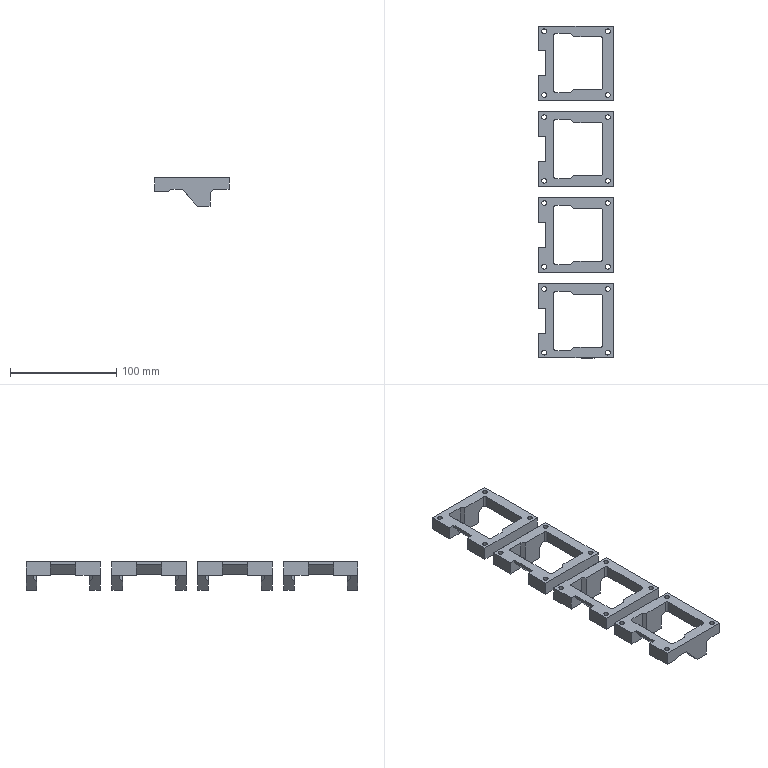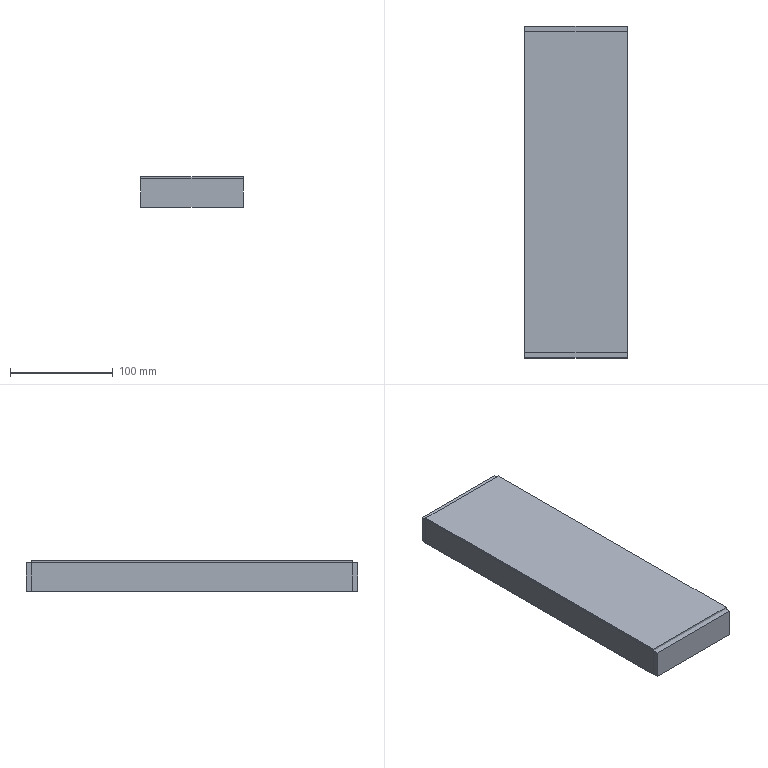CAM job | NX | 3-axis milling, drilling | part box 70 x 313 x 26.9 mm | stock box 100 x 323 x 29.9 mm
Tools:
number,name,description,diameter,corner_radius,flute_length,length,flutes
1,D63,Milling Tool-5 Parameters,63.0,0.0,50.0,75.0,2
7,D6A45,Milling Tool-5 Parameters,6.0,0.0,50.0,75.0,2
14,4.5ZT,Drilling Tool,4.5,0.0,35.0,50.0,2
10,D10,Milling Tool-5 Parameters,10.0,0.0,50.0,75.0,2
4,D4,Milling Tool-5 Parameters,4.0,0.0,50.0,75.0,2
11,D10JING,Milling Tool-5 Parameters,10.0,0.0,50.0,75.0,2
5,D4R0.5,Milling Tool-5 Parameters,4.0,0.5,50.0,75.0,2
Operations:
program,operation,operation_type,tool,method,geometry_group,spindle_rpm,surface_speed,feed_per_tooth,feed_cut,feed_plunge,cut_length_mm,path_length_mm,cut_time_min,machine_time_min
1,FLOOR_WALL,VolumeBased25DMillingOperation,D63,METHOD,A,6500.0,1286.0,0.1154,1500.0,100.0,1284.797,1338.797,0.8565,0.8619
1,CAVITY_MILL,CavityMilling,D10,METHOD,A,9500.0,298.0,0.1579,3000.0,1000.0,308716.422,324860.952,105.611,107.226
1,CAVITY_MILL_COPY_1,CavityMilling,D10JING,METHOD,A,9500.0,298.0,0.0632,1200.0,1000.0,3948.896,6181.533,3.3,3.524
1,DRILLING,Operation,D6A45,METHOD,A,5000.0,94.0,0.025,250.0,0.0,64.0,932.954,0.256,0.3429
1,DRILLING_COPY,Operation,4.5ZT,METHOD,A,2000.0,28.0,0.05,200.0,0.0,245.631,1296.216,1.228,1.333
1,CAVITY_MILL_COPY,CavityMilling,D4,METHOD,A,9500.0,119.0,0.0789,1500.0,1000.0,9181.42,17697.332,6.771,7.623
1,FLOOR_WALL_1,VolumeBased25DMillingOperation,D4,METHOD,A,9500.0,119.0,0.0658,1250.0,100.0,4950.004,9858.467,3.96,4.451
1,ZLEVEL_PROFILE,ZLevelMilling,D4R0.5,METHOD,A,9500.0,119.0,0.1579,3000.0,100.0,16650.007,17950.704,5.55,5.68
1,ZLEVEL_PROFILE_COPY,ZLevelMilling,D4R0.5,METHOD,A,9500.0,119.0,0.1579,3000.0,100.0,16899.382,17933.709,5.633,5.737
1,ZLEVEL_PROFILE_COPY_COPY,ZLevelMilling,D4R0.5,METHOD,A,9500.0,119.0,0.1579,3000.0,100.0,6480.632,9793.838,2.16,2.491
1,ZLEVEL_PROFILE_COPY_COPY_COPY,ZLevelMilling,D4R0.5,METHOD,A,9500.0,119.0,0.1579,3000.0,100.0,10578.56,11874.594,3.526,3.656
1,PLANAR_MILL,PlanarMilling,D6A45,METHOD,A,9500.0,179.0,0.0658,1250.0,100.0,325.324,997.087,0.2603,0.3274
1,PLANAR_MILL_COPY,PlanarMilling,D6A45,METHOD,A,9500.0,179.0,0.0658,1250.0,100.0,519.325,2254.248,0.4155,0.589
1,PLANAR_MILL_COPY_COPY,PlanarMilling,D6A45,METHOD,A,9500.0,179.0,0.0658,1250.0,100.0,564.468,2664.318,0.4516,0.6616
2,FLOOR_WALL_COPY,VolumeBased25DMillingOperation,D63,METHOD,B,6500.0,1286.0,0.1154,1500.0,100.0,13031.955,14427.117,8.688,8.828
2,PLANAR_MILL_COPY_1,PlanarMilling,D6A45,METHOD,B,9500.0,179.0,0.0658,1250.0,100.0,2209.153,4635.541,1.767,2.01